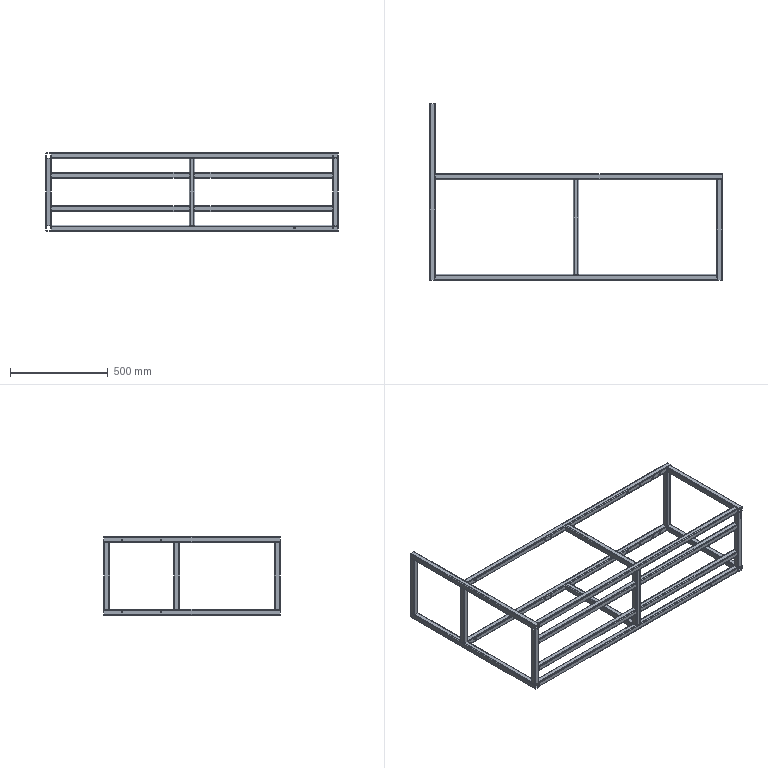Part | SolidWorks | features WeldCornerFeat 8, HoleWzd 5, 3DProfileFeature 1, ICE 1, MirrorPattern 1, WeldMemberFeat 1, WeldmentFeature 1 | 20 solids | 436 faces | box 1500 x 905 x 400 mm | volume 3870748 mm3 | cylinder 236 | plane 200 | commonest cylinder face diameters 5.2 x80 10.4 x80 9 x44 7 x16 10 x16